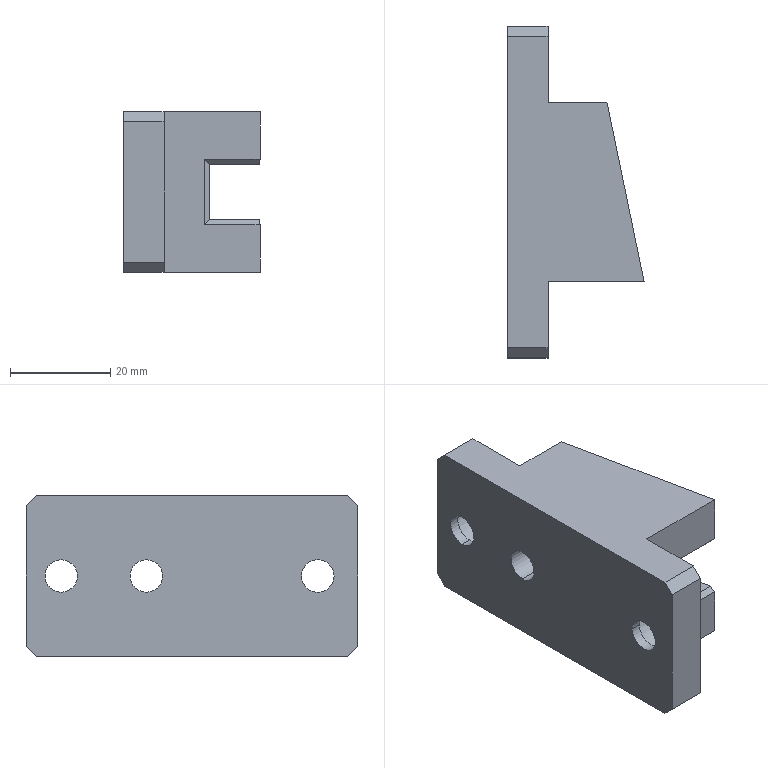Part | Creo | features CURVE 9, CUT 6, PROTRUSION 4, DATUM PLANE 3, CHAMFER 2, COORDINATE SYSTEM 1, MIRROR 1 | 1 solid | 40 faces | box 27.171 x 66.207 x 32 mm | volume 28820 mm3 | plane 28 | cylinder 12 | commonest cylinder face diameters 6.5 x6 10.5 x4 11 x2
STEP:
#1=CARTESIAN_POINT('',(0.,0.,0.));
#2=DIRECTION('',(0.,0.,1.));
#3=DIRECTION('',(1.,0.,0.));
#4=AXIS2_PLACEMENT_3D('',#1,#2,#3);
#5=CARTESIAN_POINT('',(0.,24.007,-16.));
#6=VERTEX_POINT('',#5);
#7=CARTESIAN_POINT('',(7.998,24.007,-16.));
#8=VERTEX_POINT('',#7);
#9=CARTESIAN_POINT('',(0.,24.007,-16.));
#10=DIRECTION('',(1.,0.,0.));
#11=VECTOR('',#10,7.998);
#12=LINE('',#9,#11);
#13=EDGE_CURVE('',#6,#8,#12,.T.);
#14=ORIENTED_EDGE('',*,*,#13,.F.);
#15=CARTESIAN_POINT('',(0.,-38.2,-16.));
#16=VERTEX_POINT('',#15);
#17=CARTESIAN_POINT('',(0.,24.007,-16.));
#18=DIRECTION('',(0.,-1.,0.));
#19=VECTOR('',#18,62.207);
#20=LINE('',#17,#19);
#21=EDGE_CURVE('',#6,#16,#20,.T.);
#22=ORIENTED_EDGE('',*,*,#21,.T.);
#23=CARTESIAN_POINT('',(7.998,-38.2,-16.));
#24=VERTEX_POINT('',#23);
#25=CARTESIAN_POINT('',(0.,-38.2,-16.));
#26=DIRECTION('',(1.,0.,0.));
#27=VECTOR('',#26,7.998);
#28=LINE('',#25,#27);
#29=EDGE_CURVE('',#16,#24,#28,.T.);
#30=ORIENTED_EDGE('',*,*,#29,.T.);
#31=CARTESIAN_POINT('',(7.998,-25.,-16.));
#32=VERTEX_POINT('',#31);
#33=CARTESIAN_POINT('',(7.998,-25.,-16.));
#34=DIRECTION('',(0.,-1.,0.));
#35=VECTOR('',#34,13.2);
#36=LINE('',#33,#35);
#37=EDGE_CURVE('',#32,#24,#36,.T.);
#38=ORIENTED_EDGE('',*,*,#37,.F.);
#39=CARTESIAN_POINT('',(27.171,-25.,-16.));
#40=VERTEX_POINT('',#39);
#41=CARTESIAN_POINT('',(27.171,-25.,-16.));
#42=DIRECTION('',(-1.,0.,0.));
#43=VECTOR('',#42,19.173);
#44=LINE('',#41,#43);
#45=EDGE_CURVE('',#40,#32,#44,.T.);
#46=ORIENTED_EDGE('',*,*,#45,.F.);
#47=CARTESIAN_POINT('',(19.771,10.777,-16.));
#48=VERTEX_POINT('',#47);
#49=CARTESIAN_POINT('',(27.171,-25.,-16.));
#50=DIRECTION('',(-0.2026,0.9793,0.));
#51=VECTOR('',#50,36.534);
#52=LINE('',#49,#51);
#53=EDGE_CURVE('',#40,#48,#52,.T.);
#54=ORIENTED_EDGE('',*,*,#53,.T.);
#55=CARTESIAN_POINT('',(7.998,10.777,-16.));
#56=VERTEX_POINT('',#55);
#57=CARTESIAN_POINT('',(7.998,10.777,-16.));
#58=DIRECTION('',(1.,0.,0.));
#59=VECTOR('',#58,11.773);
#60=LINE('',#57,#59);
#61=EDGE_CURVE('',#56,#48,#60,.T.);
#62=ORIENTED_EDGE('',*,*,#61,.F.);
#63=CARTESIAN_POINT('',(7.998,10.777,-16.));
#64=DIRECTION('',(0.,1.,0.));
#65=VECTOR('',#64,13.23);
#66=LINE('',#63,#65);
#67=EDGE_CURVE('',#56,#8,#66,.T.);
#68=ORIENTED_EDGE('',*,*,#67,.T.);
#69=EDGE_LOOP('',(#14,#22,#30,#38,#46,#54,#62,#68));
#70=FACE_OUTER_BOUND('',#69,.F.);
#71=CARTESIAN_POINT('',(0.,0.,-16.));
#72=DIRECTION('',(0.,0.,1.));
#73=DIRECTION('',(1.,0.,0.));
#74=AXIS2_PLACEMENT_3D('',#71,#72,#73);
#75=PLANE('',#74);
#76=ADVANCED_FACE('',(#70),#75,.F.);
#77=CARTESIAN_POINT('',(7.998,26.007,-14.));
#78=VERTEX_POINT('',#77);
#79=CARTESIAN_POINT('',(7.998,24.007,-16.));
#80=DIRECTION('',(0.,0.7071,0.7071));
#81=VECTOR('',#80,2.828);
#82=LINE('',#79,#81);
#83=EDGE_CURVE('',#8,#78,#82,.T.);
#84=ORIENTED_EDGE('',*,*,#83,.T.);
#85=CARTESIAN_POINT('',(0.,26.007,-14.));
#86=VERTEX_POINT('',#85);
#87=CARTESIAN_POINT('',(0.,26.007,-14.));
#88=DIRECTION('',(1.,0.,0.));
#89=VECTOR('',#88,7.998);
#90=LINE('',#87,#89);
#91=EDGE_CURVE('',#86,#78,#90,.T.);
#92=ORIENTED_EDGE('',*,*,#91,.F.);
#93=CARTESIAN_POINT('',(0.,26.007,-14.));
#94=DIRECTION('',(0.,-0.7071,-0.7071));
#95=VECTOR('',#94,2.828);
#96=LINE('',#93,#95);
#97=EDGE_CURVE('',#86,#6,#96,.T.);
#98=ORIENTED_EDGE('',*,*,#97,.T.);
#99=ORIENTED_EDGE('',*,*,#13,.T.);
#100=EDGE_LOOP('',(#84,#92,#98,#99));
#101=FACE_OUTER_BOUND('',#100,.F.);
#102=CARTESIAN_POINT('',(3.999,25.007,-15.));
#103=DIRECTION('',(0.,0.7071,-0.7071));
#104=DIRECTION('',(0.,0.7071,0.7071));
#105=AXIS2_PLACEMENT_3D('',#102,#103,#104);
#106=PLANE('',#105);
#107=ADVANCED_FACE('',(#101),#106,.T.);
#108=ORIENTED_EDGE('',*,*,#83,.F.);
#109=ORIENTED_EDGE('',*,*,#67,.F.);
#110=CARTESIAN_POINT('',(7.998,10.777,16.));
#111=VERTEX_POINT('',#110);
#112=CARTESIAN_POINT('',(7.998,10.777,-16.));
#113=DIRECTION('',(0.,0.,1.));
#114=VECTOR('',#113,32.);
#115=LINE('',#112,#114);
#116=EDGE_CURVE('',#56,#111,#115,.T.);
#117=ORIENTED_EDGE('',*,*,#116,.T.);
#118=CARTESIAN_POINT('',(7.998,24.007,16.));
#119=VERTEX_POINT('',#118);
#120=CARTESIAN_POINT('',(7.998,10.777,16.));
#121=DIRECTION('',(0.,1.,0.));
#122=VECTOR('',#121,13.23);
#123=LINE('',#120,#122);
#124=EDGE_CURVE('',#111,#119,#123,.T.);
#125=ORIENTED_EDGE('',*,*,#124,.T.);
#126=CARTESIAN_POINT('',(7.998,26.007,14.));
#127=VERTEX_POINT('',#126);
#128=CARTESIAN_POINT('',(7.998,26.007,14.));
#129=DIRECTION('',(0.,-0.7071,0.7071));
#130=VECTOR('',#129,2.828);
#131=LINE('',#128,#130);
#132=EDGE_CURVE('',#127,#119,#131,.T.);
#133=ORIENTED_EDGE('',*,*,#132,.F.);
#134=CARTESIAN_POINT('',(7.998,26.007,-14.));
#135=DIRECTION('',(0.,0.,1.));
#136=VECTOR('',#135,28.);
#137=LINE('',#134,#136);
#138=EDGE_CURVE('',#78,#127,#137,.T.);
#139=ORIENTED_EDGE('',*,*,#138,.F.);
#140=EDGE_LOOP('',(#108,#109,#117,#125,#133,#139));
#141=FACE_OUTER_BOUND('',#140,.F.);
#142=CARTESIAN_POINT('',(7.998,19.007,-5.25));
#143=VERTEX_POINT('',#142);
#144=CARTESIAN_POINT('',(7.998,19.007,5.25));
#145=VERTEX_POINT('',#144);
#146=CARTESIAN_POINT('',(7.998,19.007,0.));
#147=DIRECTION('',(1.,0.,0.));
#148=DIRECTION('',(0.,0.,-1.));
#149=AXIS2_PLACEMENT_3D('',#146,#147,#148);
#150=CIRCLE('',#149,5.25);
#151=EDGE_CURVE('',#143,#145,#150,.T.);
#152=ORIENTED_EDGE('',*,*,#151,.T.);
#153=CARTESIAN_POINT('',(7.998,19.007,0.));
#154=DIRECTION('',(1.,0.,0.));
#155=DIRECTION('',(0.,0.,1.));
#156=AXIS2_PLACEMENT_3D('',#153,#154,#155);
#157=CIRCLE('',#156,5.25);
#158=EDGE_CURVE('',#145,#143,#157,.T.);
#159=ORIENTED_EDGE('',*,*,#158,.T.);
#160=EDGE_LOOP('',(#152,#159));
#161=FACE_BOUND('',#160,.F.);
#162=CARTESIAN_POINT('',(7.998,10.777,-16.));
#163=DIRECTION('',(1.,0.,0.));
#164=DIRECTION('',(0.,1.,0.));
#165=AXIS2_PLACEMENT_3D('',#162,#163,#164);
#166=PLANE('',#165);
#167=ADVANCED_FACE('',(#141,#161),#166,.T.);
#168=ORIENTED_EDGE('',*,*,#151,.F.);
#169=CARTESIAN_POINT('',(1.998,19.007,-5.25));
#170=VERTEX_POINT('',#169);
#171=CARTESIAN_POINT('',(7.998,19.007,-5.25));
#172=DIRECTION('',(-1.,0.,0.));
#173=VECTOR('',#172,6.);
#174=LINE('',#171,#173);
#175=EDGE_CURVE('',#143,#170,#174,.T.);
#176=ORIENTED_EDGE('',*,*,#175,.T.);
#177=CARTESIAN_POINT('',(1.998,19.007,5.25));
#178=VERTEX_POINT('',#177);
#179=CARTESIAN_POINT('',(1.998,19.007,0.));
#180=DIRECTION('',(1.,0.,0.));
#181=DIRECTION('',(0.,0.,-1.));
#182=AXIS2_PLACEMENT_3D('',#179,#180,#181);
#183=CIRCLE('',#182,5.25);
#184=EDGE_CURVE('',#170,#178,#183,.T.);
#185=ORIENTED_EDGE('',*,*,#184,.T.);
#186=CARTESIAN_POINT('',(7.998,19.007,5.25));
#187=DIRECTION('',(-1.,0.,0.));
#188=VECTOR('',#187,6.);
#189=LINE('',#186,#188);
#190=EDGE_CURVE('',#145,#178,#189,.T.);
#191=ORIENTED_EDGE('',*,*,#190,.F.);
#192=EDGE_LOOP('',(#168,#176,#185,#191));
#193=FACE_OUTER_BOUND('',#192,.F.);
#194=CARTESIAN_POINT('',(7.998,19.007,0.));
#195=DIRECTION('',(1.,0.,0.));
#196=DIRECTION('',(0.,0.,-1.));
#197=AXIS2_PLACEMENT_3D('',#194,#195,#196);
#198=CYLINDRICAL_SURFACE('',#197,5.25);
#199=ADVANCED_FACE('',(#193),#198,.F.);
#200=ORIENTED_EDGE('',*,*,#158,.F.);
#201=ORIENTED_EDGE('',*,*,#190,.T.);
#202=CARTESIAN_POINT('',(1.998,19.007,0.));
#203=DIRECTION('',(1.,0.,0.));
#204=DIRECTION('',(0.,0.,1.));
#205=AXIS2_PLACEMENT_3D('',#202,#203,#204);
#206=CIRCLE('',#205,5.25);
#207=EDGE_CURVE('',#178,#170,#206,.T.);
#208=ORIENTED_EDGE('',*,*,#207,.T.);
#209=ORIENTED_EDGE('',*,*,#175,.F.);
#210=EDGE_LOOP('',(#200,#201,#208,#209));
#211=FACE_OUTER_BOUND('',#210,.F.);
#212=CARTESIAN_POINT('',(7.998,19.007,0.));
#213=DIRECTION('',(1.,0.,0.));
#214=DIRECTION('',(0.,0.,-1.));
#215=AXIS2_PLACEMENT_3D('',#212,#213,#214);
#216=CYLINDRICAL_SURFACE('',#215,5.25);
#217=ADVANCED_FACE('',(#211),#216,.F.);
#218=ORIENTED_EDGE('',*,*,#184,.F.);
#219=ORIENTED_EDGE('',*,*,#207,.F.);
#220=EDGE_LOOP('',(#218,#219));
#221=FACE_OUTER_BOUND('',#220,.F.);
#222=CARTESIAN_POINT('',(1.998,19.007,-3.25));
#223=VERTEX_POINT('',#222);
#224=CARTESIAN_POINT('',(1.998,19.007,3.25));
#225=VERTEX_POINT('',#224);
#226=CARTESIAN_POINT('',(1.998,19.007,0.));
#227=DIRECTION('',(1.,0.,0.));
#228=DIRECTION('',(0.,0.,-1.));
#229=AXIS2_PLACEMENT_3D('',#226,#227,#228);
#230=CIRCLE('',#229,3.25);
#231=EDGE_CURVE('',#223,#225,#230,.T.);
#232=ORIENTED_EDGE('',*,*,#231,.T.);
#233=CARTESIAN_POINT('',(1.998,19.007,0.));
#234=DIRECTION('',(1.,0.,0.));
#235=DIRECTION('',(0.,0.,1.));
#236=AXIS2_PLACEMENT_3D('',#233,#234,#235);
#237=CIRCLE('',#236,3.25);
#238=EDGE_CURVE('',#225,#223,#237,.T.);
#239=ORIENTED_EDGE('',*,*,#238,.T.);
#240=EDGE_LOOP('',(#232,#239));
#241=FACE_BOUND('',#240,.F.);
#242=CARTESIAN_POINT('',(1.998,0.,-16.));
#243=DIRECTION('',(1.,0.,0.));
#244=DIRECTION('',(0.,0.,-1.));
#245=AXIS2_PLACEMENT_3D('',#242,#243,#244);
#246=PLANE('',#245);
#247=ADVANCED_FACE('',(#221,#241),#246,.T.);
#248=ORIENTED_EDGE('',*,*,#231,.F.);
#249=CARTESIAN_POINT('',(0.,19.007,-3.25));
#250=VERTEX_POINT('',#249);
#251=CARTESIAN_POINT('',(1.998,19.007,-3.25));
#252=DIRECTION('',(-1.,0.,0.));
#253=VECTOR('',#252,1.998);
#254=LINE('',#251,#253);
#255=EDGE_CURVE('',#223,#250,#254,.T.);
#256=ORIENTED_EDGE('',*,*,#255,.T.);
#257=CARTESIAN_POINT('',(0.,19.007,3.25));
#258=VERTEX_POINT('',#257);
#259=CARTESIAN_POINT('',(0.,19.007,0.));
#260=DIRECTION('',(1.,0.,0.));
#261=DIRECTION('',(0.,0.,-1.));
#262=AXIS2_PLACEMENT_3D('',#259,#260,#261);
#263=CIRCLE('',#262,3.25);
#264=EDGE_CURVE('',#250,#258,#263,.T.);
#265=ORIENTED_EDGE('',*,*,#264,.T.);
#266=CARTESIAN_POINT('',(1.998,19.007,3.25));
#267=DIRECTION('',(-1.,0.,0.));
#268=VECTOR('',#267,1.998);
#269=LINE('',#266,#268);
#270=EDGE_CURVE('',#225,#258,#269,.T.);
#271=ORIENTED_EDGE('',*,*,#270,.F.);
#272=EDGE_LOOP('',(#248,#256,#265,#271));
#273=FACE_OUTER_BOUND('',#272,.F.);
#274=CARTESIAN_POINT('',(17.,19.007,0.));
#275=DIRECTION('',(1.,0.,0.));
#276=DIRECTION('',(0.,0.,-1.));
#277=AXIS2_PLACEMENT_3D('',#274,#275,#276);
#278=CYLINDRICAL_SURFACE('',#277,3.25);
#279=ADVANCED_FACE('',(#273),#278,.F.);
#280=ORIENTED_EDGE('',*,*,#238,.F.);
#281=ORIENTED_EDGE('',*,*,#270,.T.);
#282=CARTESIAN_POINT('',(0.,19.007,0.));
#283=DIRECTION('',(1.,0.,0.));
#284=DIRECTION('',(0.,0.,1.));
#285=AXIS2_PLACEMENT_3D('',#282,#283,#284);
#286=CIRCLE('',#285,3.25);
#287=EDGE_CURVE('',#258,#250,#286,.T.);
#288=ORIENTED_EDGE('',*,*,#287,.T.);
#289=ORIENTED_EDGE('',*,*,#255,.F.);
#290=EDGE_LOOP('',(#280,#281,#288,#289));
#291=FACE_OUTER_BOUND('',#290,.F.);
#292=CARTESIAN_POINT('',(17.,19.007,0.));
#293=DIRECTION('',(1.,0.,0.));
#294=DIRECTION('',(0.,0.,-1.));
#295=AXIS2_PLACEMENT_3D('',#292,#293,#294);
#296=CYLINDRICAL_SURFACE('',#295,3.25);
#297=ADVANCED_FACE('',(#291),#296,.F.);
#298=ORIENTED_EDGE('',*,*,#97,.F.);
#299=CARTESIAN_POINT('',(0.,26.007,14.));
#300=VERTEX_POINT('',#299);
#301=CARTESIAN_POINT('',(0.,26.007,-14.));
#302=DIRECTION('',(0.,0.,1.));
#303=VECTOR('',#302,28.);
#304=LINE('',#301,#303);
#305=EDGE_CURVE('',#86,#300,#304,.T.);
#306=ORIENTED_EDGE('',*,*,#305,.T.);
#307=CARTESIAN_POINT('',(0.,24.007,16.));
#308=VERTEX_POINT('',#307);
#309=CARTESIAN_POINT('',(0.,24.007,16.));
#310=DIRECTION('',(0.,0.7071,-0.7071));
#311=VECTOR('',#310,2.828);
#312=LINE('',#309,#311);
#313=EDGE_CURVE('',#308,#300,#312,.T.);
#314=ORIENTED_EDGE('',*,*,#313,.F.);
#315=CARTESIAN_POINT('',(0.,-38.2,16.));
#316=VERTEX_POINT('',#315);
#317=CARTESIAN_POINT('',(0.,24.007,16.));
#318=DIRECTION('',(0.,-1.,0.));
#319=VECTOR('',#318,62.207);
#320=LINE('',#317,#319);
#321=EDGE_CURVE('',#308,#316,#320,.T.);
#322=ORIENTED_EDGE('',*,*,#321,.T.);
#323=CARTESIAN_POINT('',(0.,-40.2,14.));
#324=VERTEX_POINT('',#323);
#325=CARTESIAN_POINT('',(0.,-40.2,14.));
#326=DIRECTION('',(0.,0.7071,0.7071));
#327=VECTOR('',#326,2.828);
#328=LINE('',#325,#327);
#329=EDGE_CURVE('',#324,#316,#328,.T.);
#330=ORIENTED_EDGE('',*,*,#329,.F.);
#331=CARTESIAN_POINT('',(0.,-40.2,-14.));
#332=VERTEX_POINT('',#331);
#333=CARTESIAN_POINT('',(0.,-40.2,14.));
#334=DIRECTION('',(0.,0.,-1.));
#335=VECTOR('',#334,28.);
#336=LINE('',#333,#335);
#337=EDGE_CURVE('',#324,#332,#336,.T.);
#338=ORIENTED_EDGE('',*,*,#337,.T.);
#339=CARTESIAN_POINT('',(0.,-38.2,-16.));
#340=DIRECTION('',(0.,-0.7071,0.7071));
#341=VECTOR('',#340,2.828);
#342=LINE('',#339,#341);
#343=EDGE_CURVE('',#16,#332,#342,.T.);
#344=ORIENTED_EDGE('',*,*,#343,.F.);
#345=ORIENTED_EDGE('',*,*,#21,.F.);
#346=EDGE_LOOP('',(#298,#306,#314,#322,#330,#338,#344,#345));
#347=FACE_OUTER_BOUND('',#346,.F.);
#348=CARTESIAN_POINT('',(0.,2.007,-3.25));
#349=VERTEX_POINT('',#348);
#350=CARTESIAN_POINT('',(0.,2.007,3.25));
#351=VERTEX_POINT('',#350);
#352=CARTESIAN_POINT('',(0.,2.007,0.));
#353=DIRECTION('',(1.,0.,0.));
#354=DIRECTION('',(0.,0.,-1.));
#355=AXIS2_PLACEMENT_3D('',#352,#353,#354);
#356=CIRCLE('',#355,3.25);
#357=EDGE_CURVE('',#349,#351,#356,.T.);
#358=ORIENTED_EDGE('',*,*,#357,.F.);
#359=CARTESIAN_POINT('',(0.,2.007,0.));
#360=DIRECTION('',(1.,0.,0.));
#361=DIRECTION('',(0.,0.,1.));
#362=AXIS2_PLACEMENT_3D('',#359,#360,#361);
#363=CIRCLE('',#362,3.25);
#364=EDGE_CURVE('',#351,#349,#363,.T.);
#365=ORIENTED_EDGE('',*,*,#364,.F.);
#366=EDGE_LOOP('',(#358,#365));
#367=FACE_BOUND('',#366,.F.);
#368=CARTESIAN_POINT('',(0.,-28.95,0.));
#369=VERTEX_POINT('',#368);
#370=CARTESIAN_POINT('',(0.,-35.45,0.));
#371=VERTEX_POINT('',#370);
#372=CARTESIAN_POINT('',(0.,-32.2,0.));
#373=DIRECTION('',(1.,0.,0.));
#374=DIRECTION('',(0.,1.,0.));
#375=AXIS2_PLACEMENT_3D('',#372,#373,#374);
#376=CIRCLE('',#375,3.25);
#377=EDGE_CURVE('',#369,#371,#376,.T.);
#378=ORIENTED_EDGE('',*,*,#377,.F.);
#379=CARTESIAN_POINT('',(0.,-32.2,0.));
#380=DIRECTION('',(1.,0.,0.));
#381=DIRECTION('',(0.,-1.,0.));
#382=AXIS2_PLACEMENT_3D('',#379,#380,#381);
#383=CIRCLE('',#382,3.25);
#384=EDGE_CURVE('',#371,#369,#383,.T.);
#385=ORIENTED_EDGE('',*,*,#384,.F.);
#386=EDGE_LOOP('',(#378,#385));
#387=FACE_BOUND('',#386,.F.);
#388=ORIENTED_EDGE('',*,*,#264,.F.);
#389=ORIENTED_EDGE('',*,*,#287,.F.);
#390=EDGE_LOOP('',(#388,#389));
#391=FACE_BOUND('',#390,.F.);
#392=CARTESIAN_POINT('',(0.,26.007,-16.));
#393=DIRECTION('',(-1.,0.,0.));
#394=DIRECTION('',(0.,-1.,0.));
#395=AXIS2_PLACEMENT_3D('',#392,#393,#394);
#396=PLANE('',#395);
#397=ADVANCED_FACE('',(#347,#367,#387,#391),#396,.T.);
#398=CARTESIAN_POINT('',(5.,2.007,-3.25));
#399=VERTEX_POINT('',#398);
#400=CARTESIAN_POINT('',(5.,2.007,3.25));
#401=VERTEX_POINT('',#400);
#402=CARTESIAN_POINT('',(5.,2.007,0.));
#403=DIRECTION('',(1.,0.,0.));
#404=DIRECTION('',(0.,0.,-1.));
#405=AXIS2_PLACEMENT_3D('',#402,#403,#404);
#406=CIRCLE('',#405,3.25);
#407=EDGE_CURVE('',#399,#401,#406,.T.);
#408=ORIENTED_EDGE('',*,*,#407,.F.);
#409=CARTESIAN_POINT('',(5.,2.007,-3.25));
#410=DIRECTION('',(-1.,0.,0.));
#411=VECTOR('',#410,5.);
#412=LINE('',#409,#411);
#413=EDGE_CURVE('',#399,#349,#412,.T.);
#414=ORIENTED_EDGE('',*,*,#413,.T.);
#415=ORIENTED_EDGE('',*,*,#357,.T.);
#416=CARTESIAN_POINT('',(5.,2.007,3.25));
#417=DIRECTION('',(-1.,0.,0.));
#418=VECTOR('',#417,5.);
#419=LINE('',#416,#418);
#420=EDGE_CURVE('',#401,#351,#419,.T.);
#421=ORIENTED_EDGE('',*,*,#420,.F.);
#422=EDGE_LOOP('',(#408,#414,#415,#421));
#423=FACE_OUTER_BOUND('',#422,.F.);
#424=CARTESIAN_POINT('',(17.,2.007,0.));
#425=DIRECTION('',(1.,0.,0.));
#426=DIRECTION('',(0.,0.,-1.));
#427=AXIS2_PLACEMENT_3D('',#424,#425,#426);
#428=CYLINDRICAL_SURFACE('',#427,3.25);
#429=ADVANCED_FACE('',(#423),#428,.F.);
#430=CARTESIAN_POINT('',(5.,2.007,-5.25));
#431=VERTEX_POINT('',#430);
#432=CARTESIAN_POINT('',(5.,2.007,5.25));
#433=VERTEX_POINT('',#432);
#434=CARTESIAN_POINT('',(5.,2.007,0.));
#435=DIRECTION('',(1.,0.,0.));
#436=DIRECTION('',(0.,0.,-1.));
#437=AXIS2_PLACEMENT_3D('',#434,#435,#436);
#438=CIRCLE('',#437,5.25);
#439=EDGE_CURVE('',#431,#433,#438,.T.);
#440=ORIENTED_EDGE('',*,*,#439,.F.);
#441=CARTESIAN_POINT('',(5.,2.007,0.));
#442=DIRECTION('',(1.,0.,0.));
#443=DIRECTION('',(0.,0.,1.));
#444=AXIS2_PLACEMENT_3D('',#441,#442,#443);
#445=CIRCLE('',#444,5.25);
#446=EDGE_CURVE('',#433,#431,#445,.T.);
#447=ORIENTED_EDGE('',*,*,#446,.F.);
#448=EDGE_LOOP('',(#440,#447));
#449=FACE_OUTER_BOUND('',#448,.F.);
#450=ORIENTED_EDGE('',*,*,#407,.T.);
#451=CARTESIAN_POINT('',(5.,2.007,0.));
#452=DIRECTION('',(1.,0.,0.));
#453=DIRECTION('',(0.,0.,1.));
#454=AXIS2_PLACEMENT_3D('',#451,#452,#453);
#455=CIRCLE('',#454,3.25);
#456=EDGE_CURVE('',#401,#399,#455,.T.);
#457=ORIENTED_EDGE('',*,*,#456,.T.);
#458=EDGE_LOOP('',(#450,#457));
#459=FACE_BOUND('',#458,.F.);
#460=CARTESIAN_POINT('',(5.,0.,5.5));
#461=DIRECTION('',(1.,0.,0.));
#462=DIRECTION('',(0.,0.,-1.));
#463=AXIS2_PLACEMENT_3D('',#460,#461,#462);
#464=PLANE('',#463);
#465=ADVANCED_FACE('',(#449,#459),#464,.T.);
#466=CARTESIAN_POINT('',(11.96,2.007,-5.25));
#467=VERTEX_POINT('',#466);
#468=CARTESIAN_POINT('',(11.96,2.007,5.25));
#469=VERTEX_POINT('',#468);
#470=CARTESIAN_POINT('',(11.821,2.626,-5.25));
#471=CARTESIAN_POINT('',(11.522,3.963,-5.026));
#472=CARTESIAN_POINT('',(11.174,5.517,-4.024));
#473=CARTESIAN_POINT('',(10.969,6.434,-2.889));
#474=CARTESIAN_POINT('',(10.86,6.923,-1.939));
#475=CARTESIAN_POINT('',(10.798,7.202,-0.9481));
#476=CARTESIAN_POINT('',(10.779,7.284,0.));
#477=CARTESIAN_POINT('',(10.798,7.202,0.9481));
#478=CARTESIAN_POINT('',(10.86,6.923,1.939));
#479=CARTESIAN_POINT('',(10.969,6.434,2.889));
#480=CARTESIAN_POINT('',(11.174,5.517,4.024));
#481=CARTESIAN_POINT('',(11.522,3.963,5.026));
#482=CARTESIAN_POINT('',(11.821,2.626,5.25));
#483=B_SPLINE_CURVE_WITH_KNOTS('',3,(#466,#470,#471,#472,#473,#474,#475,#476,#477,#478,#479,#480,#481,#482,#468),.UNSPECIFIED.,.F.,.F.,(4,1,1,1,1,1,1,1,1,1,1,1,4),(0.,0.125,0.25,0.3125,0.375,0.4375,0.5,0.5625,0.625,0.6875,0.75,0.875,1.),.UNSPECIFIED.);
#484=EDGE_CURVE('',#467,#469,#483,.T.);
#485=ORIENTED_EDGE('',*,*,#484,.F.);
#486=CARTESIAN_POINT('',(11.96,2.007,-5.25));
#487=DIRECTION('',(-1.,0.,0.));
#488=VECTOR('',#487,6.96);
#489=LINE('',#486,#488);
#490=EDGE_CURVE('',#467,#431,#489,.T.);
#491=ORIENTED_EDGE('',*,*,#490,.T.);
#492=ORIENTED_EDGE('',*,*,#439,.T.);
#493=CARTESIAN_POINT('',(11.96,2.007,5.25));
#494=DIRECTION('',(-1.,0.,0.));
#495=VECTOR('',#494,6.96);
#496=LINE('',#493,#495);
#497=EDGE_CURVE('',#469,#433,#496,.T.);
#498=ORIENTED_EDGE('',*,*,#497,.F.);
#499=EDGE_LOOP('',(#485,#491,#492,#498));
#500=FACE_OUTER_BOUND('',#499,.F.);
#501=CARTESIAN_POINT('',(17.,2.007,0.));
#502=DIRECTION('',(1.,0.,0.));
#503=DIRECTION('',(0.,0.,-1.));
#504=AXIS2_PLACEMENT_3D('',#501,#502,#503);
#505=CYLINDRICAL_SURFACE('',#504,5.25);
#506=ADVANCED_FACE('',(#500),#505,.F.);
#507=CARTESIAN_POINT('',(10.216,9.801,5.524));
#508=VERTEX_POINT('',#507);
#509=CARTESIAN_POINT('',(10.216,9.801,-5.524));
#510=VERTEX_POINT('',#509);
#511=CARTESIAN_POINT('',(10.216,9.801,5.524));
#512=DIRECTION('',(0.,0.,-1.));
#513=VECTOR('',#512,11.048);
#514=LINE('',#511,#513);
#515=EDGE_CURVE('',#508,#510,#514,.T.);
#516=ORIENTED_EDGE('',*,*,#515,.T.);
#517=CARTESIAN_POINT('',(10.222,9.777,-5.5));
#518=VERTEX_POINT('',#517);
#519=CARTESIAN_POINT('',(10.222,9.777,-5.5));
#520=DIRECTION('',(-0.1562,0.6984,-0.6984));
#521=VECTOR('',#520,0.03452);
#522=LINE('',#519,#521);
#523=EDGE_CURVE('',#518,#510,#522,.T.);
#524=ORIENTED_EDGE('',*,*,#523,.F.);
#525=CARTESIAN_POINT('',(17.,-20.529,-5.5));
#526=VERTEX_POINT('',#525);
#527=CARTESIAN_POINT('',(10.222,9.777,-5.5));
#528=DIRECTION('',(0.2183,-0.9759,0.));
#529=VECTOR('',#528,31.055);
#530=LINE('',#527,#529);
#531=EDGE_CURVE('',#518,#526,#530,.T.);
#532=ORIENTED_EDGE('',*,*,#531,.T.);
#533=CARTESIAN_POINT('',(17.,-20.529,5.5));
#534=VERTEX_POINT('',#533);
#535=CARTESIAN_POINT('',(17.,-20.529,5.5));
#536=DIRECTION('',(0.,0.,-1.));
#537=VECTOR('',#536,11.);
#538=LINE('',#535,#537);
#539=EDGE_CURVE('',#534,#526,#538,.T.);
#540=ORIENTED_EDGE('',*,*,#539,.F.);
#541=CARTESIAN_POINT('',(10.222,9.777,5.5));
#542=VERTEX_POINT('',#541);
#543=CARTESIAN_POINT('',(10.222,9.777,5.5));
#544=DIRECTION('',(0.2183,-0.9759,0.));
#545=VECTOR('',#544,31.055);
#546=LINE('',#543,#545);
#547=EDGE_CURVE('',#542,#534,#546,.T.);
#548=ORIENTED_EDGE('',*,*,#547,.F.);
#549=CARTESIAN_POINT('',(10.216,9.801,5.524));
#550=DIRECTION('',(0.1562,-0.6984,-0.6984));
#551=VECTOR('',#550,0.03452);
#552=LINE('',#549,#551);
#553=EDGE_CURVE('',#508,#542,#552,.T.);
#554=ORIENTED_EDGE('',*,*,#553,.F.);
#555=EDGE_LOOP('',(#516,#524,#532,#540,#548,#554));
#556=FACE_OUTER_BOUND('',#555,.F.);
#557=ORIENTED_EDGE('',*,*,#484,.T.);
#558=CARTESIAN_POINT('',(11.96,2.007,5.25));
#559=CARTESIAN_POINT('',(12.098,1.388,5.25));
#560=CARTESIAN_POINT('',(12.397,0.05091,5.026));
#561=CARTESIAN_POINT('',(12.745,-1.503,4.024));
#562=CARTESIAN_POINT('',(12.95,-2.42,2.889));
#563=CARTESIAN_POINT('',(13.059,-2.91,1.939));
#564=CARTESIAN_POINT('',(13.121,-3.188,0.9481));
#565=CARTESIAN_POINT('',(13.14,-3.271,0.));
#566=CARTESIAN_POINT('',(13.121,-3.188,-0.9481));
#567=CARTESIAN_POINT('',(13.059,-2.91,-1.939));
#568=CARTESIAN_POINT('',(12.95,-2.42,-2.889));
#569=CARTESIAN_POINT('',(12.745,-1.503,-4.024));
#570=CARTESIAN_POINT('',(12.397,0.05091,-5.026));
#571=CARTESIAN_POINT('',(12.098,1.388,-5.25));
#572=CARTESIAN_POINT('',(11.96,2.007,-5.25));
#573=B_SPLINE_CURVE_WITH_KNOTS('',3,(#558,#559,#560,#561,#562,#563,#564,#565,#566,#567,#568,#569,#570,#571,#572),.UNSPECIFIED.,.F.,.F.,(4,1,1,1,1,1,1,1,1,1,1,1,4),(0.,0.125,0.25,0.3125,0.375,0.4375,0.5,0.5625,0.625,0.6875,0.75,0.875,1.),.UNSPECIFIED.);
#574=EDGE_CURVE('',#469,#467,#573,.T.);
#575=ORIENTED_EDGE('',*,*,#574,.T.);
#576=EDGE_LOOP('',(#557,#575));
#577=FACE_BOUND('',#576,.F.);
#578=CARTESIAN_POINT('',(9.998,10.777,5.5));
#579=DIRECTION('',(-0.9759,-0.2183,0.));
#580=DIRECTION('',(0.2183,-0.9759,0.));
#581=AXIS2_PLACEMENT_3D('',#578,#579,#580);
#582=PLANE('',#581);
#583=ADVANCED_FACE('',(#556,#577),#582,.F.);
#584=ORIENTED_EDGE('',*,*,#574,.F.);
#585=ORIENTED_EDGE('',*,*,#497,.T.);
#586=ORIENTED_EDGE('',*,*,#446,.T.);
#587=ORIENTED_EDGE('',*,*,#490,.F.);
#588=EDGE_LOOP('',(#584,#585,#586,#587));
#589=FACE_OUTER_BOUND('',#588,.F.);
#590=CARTESIAN_POINT('',(17.,2.007,0.));
#591=DIRECTION('',(1.,0.,0.));
#592=DIRECTION('',(0.,0.,-1.));
#593=AXIS2_PLACEMENT_3D('',#590,#591,#592);
#594=CYLINDRICAL_SURFACE('',#593,5.25);
#595=ADVANCED_FACE('',(#589),#594,.F.);
#596=ORIENTED_EDGE('',*,*,#515,.F.);
#597=CARTESIAN_POINT('',(8.998,10.777,6.5));
#598=VERTEX_POINT('',#597);
#599=CARTESIAN_POINT('',(10.216,9.801,5.524));
#600=DIRECTION('',(-0.6618,0.5301,0.5301));
#601=VECTOR('',#600,1.841);
#602=LINE('',#599,#601);
#603=EDGE_CURVE('',#508,#598,#602,.T.);
#604=ORIENTED_EDGE('',*,*,#603,.T.);
#605=CARTESIAN_POINT('',(8.998,10.777,-6.5));
#606=VERTEX_POINT('',#605);
#607=CARTESIAN_POINT('',(8.998,10.777,6.5));
#608=DIRECTION('',(0.,0.,-1.));
#609=VECTOR('',#608,13.);
#610=LINE('',#607,#609);
#611=EDGE_CURVE('',#598,#606,#610,.T.);
#612=ORIENTED_EDGE('',*,*,#611,.T.);
#613=CARTESIAN_POINT('',(10.216,9.801,-5.524));
#614=DIRECTION('',(-0.6618,0.5301,-0.5301));
#615=VECTOR('',#614,1.841);
#616=LINE('',#613,#615);
#617=EDGE_CURVE('',#510,#606,#616,.T.);
#618=ORIENTED_EDGE('',*,*,#617,.F.);
#619=EDGE_LOOP('',(#596,#604,#612,#618));
#620=FACE_OUTER_BOUND('',#619,.F.);
#621=CARTESIAN_POINT('',(9.607,10.289,0.));
#622=DIRECTION('',(0.6252,0.7805,0.));
#623=DIRECTION('',(0.7805,-0.6252,0.));
#624=AXIS2_PLACEMENT_3D('',#621,#622,#623);
#625=PLANE('',#624);
#626=ADVANCED_FACE('',(#620),#625,.T.);
#627=CARTESIAN_POINT('',(19.977,9.777,5.5));
#628=VERTEX_POINT('',#627);
#629=CARTESIAN_POINT('',(19.771,10.777,6.5));
#630=VERTEX_POINT('',#629);
#631=CARTESIAN_POINT('',(19.977,9.777,5.5));
#632=DIRECTION('',(-0.1447,0.6997,0.6997));
#633=VECTOR('',#632,1.429);
#634=LINE('',#631,#633);
#635=EDGE_CURVE('',#628,#630,#634,.T.);
#636=ORIENTED_EDGE('',*,*,#635,.T.);
#637=CARTESIAN_POINT('',(19.771,10.777,6.5));
#638=DIRECTION('',(-1.,0.,0.));
#639=VECTOR('',#638,10.773);
#640=LINE('',#637,#639);
#641=EDGE_CURVE('',#630,#598,#640,.T.);
#642=ORIENTED_EDGE('',*,*,#641,.T.);
#643=ORIENTED_EDGE('',*,*,#603,.F.);
#644=ORIENTED_EDGE('',*,*,#553,.T.);
#645=CARTESIAN_POINT('',(19.977,9.777,5.5));
#646=DIRECTION('',(-1.,0.,0.));
#647=VECTOR('',#646,9.756);
#648=LINE('',#645,#647);
#649=EDGE_CURVE('',#628,#542,#648,.T.);
#650=ORIENTED_EDGE('',*,*,#649,.F.);
#651=EDGE_LOOP('',(#636,#642,#643,#644,#650));
#652=FACE_OUTER_BOUND('',#651,.F.);
#653=CARTESIAN_POINT('',(14.996,10.277,6.));
#654=DIRECTION('',(0.,0.7071,-0.7071));
#655=DIRECTION('',(0.,-0.7071,-0.7071));
#656=AXIS2_PLACEMENT_3D('',#653,#654,#655);
#657=PLANE('',#656);
#658=ADVANCED_FACE('',(#652),#657,.T.);
#659=CARTESIAN_POINT('',(27.171,-25.,6.5));
#660=VERTEX_POINT('',#659);
#661=CARTESIAN_POINT('',(26.964,-24.,5.5));
#662=VERTEX_POINT('',#661);
#663=CARTESIAN_POINT('',(27.171,-25.,6.5));
#664=DIRECTION('',(-0.1447,0.6997,-0.6997));
#665=VECTOR('',#664,1.429);
#666=LINE('',#663,#665);
#667=EDGE_CURVE('',#660,#662,#666,.T.);
#668=ORIENTED_EDGE('',*,*,#667,.F.);
#669=CARTESIAN_POINT('',(27.171,-25.,16.));
#670=VERTEX_POINT('',#669);
#671=CARTESIAN_POINT('',(27.171,-25.,16.));
#672=DIRECTION('',(0.,0.,-1.));
#673=VECTOR('',#672,9.5);
#674=LINE('',#671,#673);
#675=EDGE_CURVE('',#670,#660,#674,.T.);
#676=ORIENTED_EDGE('',*,*,#675,.F.);
#677=CARTESIAN_POINT('',(19.771,10.777,16.));
#678=VERTEX_POINT('',#677);
#679=CARTESIAN_POINT('',(27.171,-25.,16.));
#680=DIRECTION('',(-0.2026,0.9793,0.));
#681=VECTOR('',#680,36.534);
#682=LINE('',#679,#681);
#683=EDGE_CURVE('',#670,#678,#682,.T.);
#684=ORIENTED_EDGE('',*,*,#683,.T.);
#685=CARTESIAN_POINT('',(19.771,10.777,16.));
#686=DIRECTION('',(0.,0.,-1.));
#687=VECTOR('',#686,9.5);
#688=LINE('',#685,#687);
#689=EDGE_CURVE('',#678,#630,#688,.T.);
#690=ORIENTED_EDGE('',*,*,#689,.T.);
#691=ORIENTED_EDGE('',*,*,#635,.F.);
#692=CARTESIAN_POINT('',(26.964,-24.,5.5));
#693=DIRECTION('',(-0.2026,0.9793,0.));
#694=VECTOR('',#693,34.492);
#695=LINE('',#692,#694);
#696=EDGE_CURVE('',#662,#628,#695,.T.);
#697=ORIENTED_EDGE('',*,*,#696,.F.);
#698=EDGE_LOOP('',(#668,#676,#684,#690,#691,#697));
#699=FACE_OUTER_BOUND('',#698,.F.);
#700=CARTESIAN_POINT('',(27.171,-25.,16.));
#701=DIRECTION('',(0.9793,0.2026,0.));
#702=DIRECTION('',(-0.2026,0.9793,0.));
#703=AXIS2_PLACEMENT_3D('',#700,#701,#702);
#704=PLANE('',#703);
#705=ADVANCED_FACE('',(#699),#704,.T.);
#706=ORIENTED_EDGE('',*,*,#667,.T.);
#707=CARTESIAN_POINT('',(17.,-24.,5.5));
#708=VERTEX_POINT('',#707);
#709=CARTESIAN_POINT('',(17.,-24.,5.5));
#710=DIRECTION('',(1.,0.,0.));
#711=VECTOR('',#710,9.964);
#712=LINE('',#709,#711);
#713=EDGE_CURVE('',#708,#662,#712,.T.);
#714=ORIENTED_EDGE('',*,*,#713,.F.);
#715=CARTESIAN_POINT('',(16.,-25.,6.5));
#716=VERTEX_POINT('',#715);
#717=CARTESIAN_POINT('',(17.,-24.,5.5));
#718=DIRECTION('',(-0.5774,-0.5774,0.5774));
#719=VECTOR('',#718,1.732);
#720=LINE('',#717,#719);
#721=EDGE_CURVE('',#708,#716,#720,.T.);
#722=ORIENTED_EDGE('',*,*,#721,.T.);
#723=CARTESIAN_POINT('',(16.,-25.,6.5));
#724=DIRECTION('',(1.,0.,0.));
#725=VECTOR('',#724,11.171);
#726=LINE('',#723,#725);
#727=EDGE_CURVE('',#716,#660,#726,.T.);
#728=ORIENTED_EDGE('',*,*,#727,.T.);
#729=EDGE_LOOP('',(#706,#714,#722,#728));
#730=FACE_OUTER_BOUND('',#729,.F.);
#731=CARTESIAN_POINT('',(21.982,-24.5,6.));
#732=DIRECTION('',(0.,-0.7071,-0.7071));
#733=DIRECTION('',(0.,0.7071,-0.7071));
#734=AXIS2_PLACEMENT_3D('',#731,#732,#733);
#735=PLANE('',#734);
#736=ADVANCED_FACE('',(#730),#735,.T.);
#737=ORIENTED_EDGE('',*,*,#713,.T.);
#738=ORIENTED_EDGE('',*,*,#696,.T.);
#739=ORIENTED_EDGE('',*,*,#649,.T.);
#740=ORIENTED_EDGE('',*,*,#547,.T.);
#741=CARTESIAN_POINT('',(17.,-20.529,5.5));
#742=DIRECTION('',(0.,-1.,0.));
#743=VECTOR('',#742,3.471);
#744=LINE('',#741,#743);
#745=EDGE_CURVE('',#534,#708,#744,.T.);
#746=ORIENTED_EDGE('',*,*,#745,.T.);
#747=EDGE_LOOP('',(#737,#738,#739,#740,#746));
#748=FACE_OUTER_BOUND('',#747,.F.);
#749=CARTESIAN_POINT('',(0.,0.,5.5));
#750=DIRECTION('',(0.,0.,1.));
#751=DIRECTION('',(1.,0.,0.));
#752=AXIS2_PLACEMENT_3D('',#749,#750,#751);
#753=PLANE('',#752);
#754=ADVANCED_FACE('',(#748),#753,.F.);
#755=CARTESIAN_POINT('',(17.,-24.,-5.5));
#756=VERTEX_POINT('',#755);
#757=CARTESIAN_POINT('',(17.,-24.,-5.5));
#758=DIRECTION('',(0.,0.,1.));
#759=VECTOR('',#758,11.);
#760=LINE('',#757,#759);
#761=EDGE_CURVE('',#756,#708,#760,.T.);
#762=ORIENTED_EDGE('',*,*,#761,.T.);
#763=ORIENTED_EDGE('',*,*,#745,.F.);
#764=ORIENTED_EDGE('',*,*,#539,.T.);
#765=CARTESIAN_POINT('',(17.,-20.529,-5.5));
#766=DIRECTION('',(0.,-1.,0.));
#767=VECTOR('',#766,3.471);
#768=LINE('',#765,#767);
#769=EDGE_CURVE('',#526,#756,#768,.T.);
#770=ORIENTED_EDGE('',*,*,#769,.T.);
#771=EDGE_LOOP('',(#762,#763,#764,#770));
#772=FACE_OUTER_BOUND('',#771,.F.);
#773=CARTESIAN_POINT('',(17.,-20.529,5.5));
#774=DIRECTION('',(-1.,0.,0.));
#775=DIRECTION('',(0.,-1.,0.));
#776=AXIS2_PLACEMENT_3D('',#773,#774,#775);
#777=PLANE('',#776);
#778=ADVANCED_FACE('',(#772),#777,.F.);
#779=CARTESIAN_POINT('',(16.,-25.,-6.5));
#780=VERTEX_POINT('',#779);
#781=CARTESIAN_POINT('',(16.,-25.,-6.5));
#782=DIRECTION('',(0.,0.,1.));
#783=VECTOR('',#782,13.);
#784=LINE('',#781,#783);
#785=EDGE_CURVE('',#780,#716,#784,.T.);
#786=ORIENTED_EDGE('',*,*,#785,.T.);
#787=ORIENTED_EDGE('',*,*,#721,.F.);
#788=ORIENTED_EDGE('',*,*,#761,.F.);
#789=CARTESIAN_POINT('',(17.,-24.,-5.5));
#790=DIRECTION('',(-0.5774,-0.5774,-0.5774));
#791=VECTOR('',#790,1.732);
#792=LINE('',#789,#791);
#793=EDGE_CURVE('',#756,#780,#792,.T.);
#794=ORIENTED_EDGE('',*,*,#793,.T.);
#795=EDGE_LOOP('',(#786,#787,#788,#794));
#796=FACE_OUTER_BOUND('',#795,.F.);
#797=CARTESIAN_POINT('',(16.5,-24.5,0.));
#798=DIRECTION('',(0.7071,-0.7071,0.));
#799=DIRECTION('',(0.7071,0.7071,0.));
#800=AXIS2_PLACEMENT_3D('',#797,#798,#799);
#801=PLANE('',#800);
#802=ADVANCED_FACE('',(#796),#801,.T.);
#803=CARTESIAN_POINT('',(7.998,-25.,16.));
#804=VERTEX_POINT('',#803);
#805=CARTESIAN_POINT('',(7.998,-25.,-16.));
#806=DIRECTION('',(0.,0.,1.));
#807=VECTOR('',#806,32.);
#808=LINE('',#805,#807);
#809=EDGE_CURVE('',#32,#804,#808,.T.);
#810=ORIENTED_EDGE('',*,*,#809,.T.);
#811=CARTESIAN_POINT('',(7.998,-25.,16.));
#812=DIRECTION('',(1.,0.,0.));
#813=VECTOR('',#812,19.173);
#814=LINE('',#811,#813);
#815=EDGE_CURVE('',#804,#670,#814,.T.);
#816=ORIENTED_EDGE('',*,*,#815,.T.);
#817=ORIENTED_EDGE('',*,*,#675,.T.);
#818=ORIENTED_EDGE('',*,*,#727,.F.);
#819=ORIENTED_EDGE('',*,*,#785,.F.);
#820=CARTESIAN_POINT('',(27.171,-25.,-6.5));
#821=VERTEX_POINT('',#820);
#822=CARTESIAN_POINT('',(27.171,-25.,-6.5));
#823=DIRECTION('',(-1.,0.,0.));
#824=VECTOR('',#823,11.171);
#825=LINE('',#822,#824);
#826=EDGE_CURVE('',#821,#780,#825,.T.);
#827=ORIENTED_EDGE('',*,*,#826,.F.);
#828=CARTESIAN_POINT('',(27.171,-25.,-16.));
#829=DIRECTION('',(0.,0.,1.));
#830=VECTOR('',#829,9.5);
#831=LINE('',#828,#830);
#832=EDGE_CURVE('',#40,#821,#831,.T.);
#833=ORIENTED_EDGE('',*,*,#832,.F.);
#834=ORIENTED_EDGE('',*,*,#45,.T.);
#835=EDGE_LOOP('',(#810,#816,#817,#818,#819,#827,#833,#834));
#836=FACE_OUTER_BOUND('',#835,.F.);
#837=CARTESIAN_POINT('',(0.,-25.,-16.));
#838=DIRECTION('',(0.,-1.,0.));
#839=DIRECTION('',(1.,0.,0.));
#840=AXIS2_PLACEMENT_3D('',#837,#838,#839);
#841=PLANE('',#840);
#842=ADVANCED_FACE('',(#836),#841,.T.);
#843=CARTESIAN_POINT('',(7.998,-38.2,16.));
#844=VERTEX_POINT('',#843);
#845=CARTESIAN_POINT('',(7.998,-40.2,14.));
#846=VERTEX_POINT('',#845);
#847=CARTESIAN_POINT('',(7.998,-38.2,16.));
#848=DIRECTION('',(0.,-0.7071,-0.7071));
#849=VECTOR('',#848,2.828);
#850=LINE('',#847,#849);
#851=EDGE_CURVE('',#844,#846,#850,.T.);
#852=ORIENTED_EDGE('',*,*,#851,.F.);
#853=CARTESIAN_POINT('',(7.998,-25.,16.));
#854=DIRECTION('',(0.,-1.,0.));
#855=VECTOR('',#854,13.2);
#856=LINE('',#853,#855);
#857=EDGE_CURVE('',#804,#844,#856,.T.);
#858=ORIENTED_EDGE('',*,*,#857,.F.);
#859=ORIENTED_EDGE('',*,*,#809,.F.);
#860=ORIENTED_EDGE('',*,*,#37,.T.);
#861=CARTESIAN_POINT('',(7.998,-40.2,-14.));
#862=VERTEX_POINT('',#861);
#863=CARTESIAN_POINT('',(7.998,-40.2,-14.));
#864=DIRECTION('',(0.,0.7071,-0.7071));
#865=VECTOR('',#864,2.828);
#866=LINE('',#863,#865);
#867=EDGE_CURVE('',#862,#24,#866,.T.);
#868=ORIENTED_EDGE('',*,*,#867,.F.);
#869=CARTESIAN_POINT('',(7.998,-40.2,-14.));
#870=DIRECTION('',(0.,0.,1.));
#871=VECTOR('',#870,28.);
#872=LINE('',#869,#871);
#873=EDGE_CURVE('',#862,#846,#872,.T.);
#874=ORIENTED_EDGE('',*,*,#873,.T.);
#875=EDGE_LOOP('',(#852,#858,#859,#860,#868,#874));
#876=FACE_OUTER_BOUND('',#875,.F.);
#877=CARTESIAN_POINT('',(7.998,-26.7,0.));
#878=VERTEX_POINT('',#877);
#879=CARTESIAN_POINT('',(7.998,-37.7,0.));
#880=VERTEX_POINT('',#879);
#881=CARTESIAN_POINT('',(7.998,-32.2,0.));
#882=DIRECTION('',(1.,0.,0.));
#883=DIRECTION('',(0.,1.,0.));
#884=AXIS2_PLACEMENT_3D('',#881,#882,#883);
#885=CIRCLE('',#884,5.5);
#886=EDGE_CURVE('',#878,#880,#885,.T.);
#887=ORIENTED_EDGE('',*,*,#886,.T.);
#888=CARTESIAN_POINT('',(7.998,-32.2,0.));
#889=DIRECTION('',(1.,0.,0.));
#890=DIRECTION('',(0.,-1.,0.));
#891=AXIS2_PLACEMENT_3D('',#888,#889,#890);
#892=CIRCLE('',#891,5.5);
#893=EDGE_CURVE('',#880,#878,#892,.T.);
#894=ORIENTED_EDGE('',*,*,#893,.T.);
#895=EDGE_LOOP('',(#887,#894));
#896=FACE_BOUND('',#895,.F.);
#897=CARTESIAN_POINT('',(7.998,-25.,-16.));
#898=DIRECTION('',(1.,0.,0.));
#899=DIRECTION('',(0.,0.,1.));
#900=AXIS2_PLACEMENT_3D('',#897,#898,#899);
#901=PLANE('',#900);
#902=ADVANCED_FACE('',(#876,#896),#901,.T.);
#903=ORIENTED_EDGE('',*,*,#886,.F.);
#904=CARTESIAN_POINT('',(1.998,-26.7,0.));
#905=VERTEX_POINT('',#904);
#906=CARTESIAN_POINT('',(7.998,-26.7,0.));
#907=DIRECTION('',(-1.,0.,0.));
#908=VECTOR('',#907,6.);
#909=LINE('',#906,#908);
#910=EDGE_CURVE('',#878,#905,#909,.T.);
#911=ORIENTED_EDGE('',*,*,#910,.T.);
#912=CARTESIAN_POINT('',(1.998,-37.7,0.));
#913=VERTEX_POINT('',#912);
#914=CARTESIAN_POINT('',(1.998,-32.2,0.));
#915=DIRECTION('',(1.,0.,0.));
#916=DIRECTION('',(0.,1.,0.));
#917=AXIS2_PLACEMENT_3D('',#914,#915,#916);
#918=CIRCLE('',#917,5.5);
#919=EDGE_CURVE('',#905,#913,#918,.T.);
#920=ORIENTED_EDGE('',*,*,#919,.T.);
#921=CARTESIAN_POINT('',(7.998,-37.7,0.));
#922=DIRECTION('',(-1.,0.,0.));
#923=VECTOR('',#922,6.);
#924=LINE('',#921,#923);
#925=EDGE_CURVE('',#880,#913,#924,.T.);
#926=ORIENTED_EDGE('',*,*,#925,.F.);
#927=EDGE_LOOP('',(#903,#911,#920,#926));
#928=FACE_OUTER_BOUND('',#927,.F.);
#929=CARTESIAN_POINT('',(7.998,-32.2,0.));
#930=DIRECTION('',(1.,0.,0.));
#931=DIRECTION('',(0.,1.,0.));
#932=AXIS2_PLACEMENT_3D('',#929,#930,#931);
#933=CYLINDRICAL_SURFACE('',#932,5.5);
#934=ADVANCED_FACE('',(#928),#933,.F.);
#935=ORIENTED_EDGE('',*,*,#893,.F.);
#936=ORIENTED_EDGE('',*,*,#925,.T.);
#937=CARTESIAN_POINT('',(1.998,-32.2,0.));
#938=DIRECTION('',(1.,0.,0.));
#939=DIRECTION('',(0.,-1.,0.));
#940=AXIS2_PLACEMENT_3D('',#937,#938,#939);
#941=CIRCLE('',#940,5.5);
#942=EDGE_CURVE('',#913,#905,#941,.T.);
#943=ORIENTED_EDGE('',*,*,#942,.T.);
#944=ORIENTED_EDGE('',*,*,#910,.F.);
#945=EDGE_LOOP('',(#935,#936,#943,#944));
#946=FACE_OUTER_BOUND('',#945,.F.);
#947=CARTESIAN_POINT('',(7.998,-32.2,0.));
#948=DIRECTION('',(1.,0.,0.));
#949=DIRECTION('',(0.,1.,0.));
#950=AXIS2_PLACEMENT_3D('',#947,#948,#949);
#951=CYLINDRICAL_SURFACE('',#950,5.5);
#952=ADVANCED_FACE('',(#946),#951,.F.);
#953=ORIENTED_EDGE('',*,*,#919,.F.);
#954=ORIENTED_EDGE('',*,*,#942,.F.);
#955=EDGE_LOOP('',(#953,#954));
#956=FACE_OUTER_BOUND('',#955,.F.);
#957=CARTESIAN_POINT('',(1.998,-28.95,0.));
#958=VERTEX_POINT('',#957);
#959=CARTESIAN_POINT('',(1.998,-35.45,0.));
#960=VERTEX_POINT('',#959);
#961=CARTESIAN_POINT('',(1.998,-32.2,0.));
#962=DIRECTION('',(1.,0.,0.));
#963=DIRECTION('',(0.,1.,0.));
#964=AXIS2_PLACEMENT_3D('',#961,#962,#963);
#965=CIRCLE('',#964,3.25);
#966=EDGE_CURVE('',#958,#960,#965,.T.);
#967=ORIENTED_EDGE('',*,*,#966,.T.);
#968=CARTESIAN_POINT('',(1.998,-32.2,0.));
#969=DIRECTION('',(1.,0.,0.));
#970=DIRECTION('',(0.,-1.,0.));
#971=AXIS2_PLACEMENT_3D('',#968,#969,#970);
#972=CIRCLE('',#971,3.25);
#973=EDGE_CURVE('',#960,#958,#972,.T.);
#974=ORIENTED_EDGE('',*,*,#973,.T.);
#975=EDGE_LOOP('',(#967,#974));
#976=FACE_BOUND('',#975,.F.);
#977=CARTESIAN_POINT('',(1.998,-40.2,-16.));
#978=DIRECTION('',(1.,0.,0.));
#979=DIRECTION('',(0.,1.,0.));
#980=AXIS2_PLACEMENT_3D('',#977,#978,#979);
#981=PLANE('',#980);
#982=ADVANCED_FACE('',(#956,#976),#981,.T.);
#983=ORIENTED_EDGE('',*,*,#377,.T.);
#984=CARTESIAN_POINT('',(1.998,-35.45,0.));
#985=DIRECTION('',(-1.,0.,0.));
#986=VECTOR('',#985,1.998);
#987=LINE('',#984,#986);
#988=EDGE_CURVE('',#960,#371,#987,.T.);
#989=ORIENTED_EDGE('',*,*,#988,.F.);
#990=ORIENTED_EDGE('',*,*,#966,.F.);
#991=CARTESIAN_POINT('',(1.998,-28.95,0.));
#992=DIRECTION('',(-1.,0.,0.));
#993=VECTOR('',#992,1.998);
#994=LINE('',#991,#993);
#995=EDGE_CURVE('',#958,#369,#994,.T.);
#996=ORIENTED_EDGE('',*,*,#995,.T.);
#997=EDGE_LOOP('',(#983,#989,#990,#996));
#998=FACE_OUTER_BOUND('',#997,.F.);
#999=CARTESIAN_POINT('',(7.998,-32.2,0.));
#1000=DIRECTION('',(1.,0.,0.));
#1001=DIRECTION('',(0.,1.,0.));
#1002=AXIS2_PLACEMENT_3D('',#999,#1000,#1001);
#1003=CYLINDRICAL_SURFACE('',#1002,3.25);
#1004=ADVANCED_FACE('',(#998),#1003,.F.);
#1005=ORIENTED_EDGE('',*,*,#384,.T.);
#1006=ORIENTED_EDGE('',*,*,#995,.F.);
#1007=ORIENTED_EDGE('',*,*,#973,.F.);
#1008=ORIENTED_EDGE('',*,*,#988,.T.);
#1009=EDGE_LOOP('',(#1005,#1006,#1007,#1008));
#1010=FACE_OUTER_BOUND('',#1009,.F.);
#1011=CARTESIAN_POINT('',(7.998,-32.2,0.));
#1012=DIRECTION('',(1.,0.,0.));
#1013=DIRECTION('',(0.,1.,0.));
#1014=AXIS2_PLACEMENT_3D('',#1011,#1012,#1013);
#1015=CYLINDRICAL_SURFACE('',#1014,3.25);
#1016=ADVANCED_FACE('',(#1010),#1015,.F.);
#1017=ORIENTED_EDGE('',*,*,#329,.T.);
#1018=CARTESIAN_POINT('',(7.998,-38.2,16.));
#1019=DIRECTION('',(-1.,0.,0.));
#1020=VECTOR('',#1019,7.998);
#1021=LINE('',#1018,#1020);
#1022=EDGE_CURVE('',#844,#316,#1021,.T.);
#1023=ORIENTED_EDGE('',*,*,#1022,.F.);
#1024=ORIENTED_EDGE('',*,*,#851,.T.);
#1025=CARTESIAN_POINT('',(7.998,-40.2,14.));
#1026=DIRECTION('',(-1.,0.,0.));
#1027=VECTOR('',#1026,7.998);
#1028=LINE('',#1025,#1027);
#1029=EDGE_CURVE('',#846,#324,#1028,.T.);
#1030=ORIENTED_EDGE('',*,*,#1029,.T.);
#1031=EDGE_LOOP('',(#1017,#1023,#1024,#1030));
#1032=FACE_OUTER_BOUND('',#1031,.F.);
#1033=CARTESIAN_POINT('',(3.999,-39.2,15.));
#1034=DIRECTION('',(0.,-0.7071,0.7071));
#1035=DIRECTION('',(0.,0.7071,0.7071));
#1036=AXIS2_PLACEMENT_3D('',#1033,#1034,#1035);
#1037=PLANE('',#1036);
#1038=ADVANCED_FACE('',(#1032),#1037,.T.);
#1039=CARTESIAN_POINT('',(7.998,24.007,16.));
#1040=DIRECTION('',(-1.,0.,0.));
#1041=VECTOR('',#1040,7.998);
#1042=LINE('',#1039,#1041);
#1043=EDGE_CURVE('',#119,#308,#1042,.T.);
#1044=ORIENTED_EDGE('',*,*,#1043,.F.);
#1045=ORIENTED_EDGE('',*,*,#124,.F.);
#1046=CARTESIAN_POINT('',(19.771,10.777,16.));
#1047=DIRECTION('',(-1.,0.,0.));
#1048=VECTOR('',#1047,11.773);
#1049=LINE('',#1046,#1048);
#1050=EDGE_CURVE('',#678,#111,#1049,.T.);
#1051=ORIENTED_EDGE('',*,*,#1050,.F.);
#1052=ORIENTED_EDGE('',*,*,#683,.F.);
#1053=ORIENTED_EDGE('',*,*,#815,.F.);
#1054=ORIENTED_EDGE('',*,*,#857,.T.);
#1055=ORIENTED_EDGE('',*,*,#1022,.T.);
#1056=ORIENTED_EDGE('',*,*,#321,.F.);
#1057=EDGE_LOOP('',(#1044,#1045,#1051,#1052,#1053,#1054,#1055,#1056));
#1058=FACE_OUTER_BOUND('',#1057,.F.);
#1059=CARTESIAN_POINT('',(0.,0.,16.));
#1060=DIRECTION('',(0.,0.,1.));
#1061=DIRECTION('',(1.,0.,0.));
#1062=AXIS2_PLACEMENT_3D('',#1059,#1060,#1061);
#1063=PLANE('',#1062);
#1064=ADVANCED_FACE('',(#1058),#1063,.T.);
#1065=ORIENTED_EDGE('',*,*,#313,.T.);
#1066=CARTESIAN_POINT('',(7.998,26.007,14.));
#1067=DIRECTION('',(-1.,0.,0.));
#1068=VECTOR('',#1067,7.998);
#1069=LINE('',#1066,#1068);
#1070=EDGE_CURVE('',#127,#300,#1069,.T.);
#1071=ORIENTED_EDGE('',*,*,#1070,.F.);
#1072=ORIENTED_EDGE('',*,*,#132,.T.);
#1073=ORIENTED_EDGE('',*,*,#1043,.T.);
#1074=EDGE_LOOP('',(#1065,#1071,#1072,#1073));
#1075=FACE_OUTER_BOUND('',#1074,.F.);
#1076=CARTESIAN_POINT('',(3.999,25.007,15.));
#1077=DIRECTION('',(0.,0.7071,0.7071));
#1078=DIRECTION('',(0.,0.7071,-0.7071));
#1079=AXIS2_PLACEMENT_3D('',#1076,#1077,#1078);
#1080=PLANE('',#1079);
#1081=ADVANCED_FACE('',(#1075),#1080,.T.);
#1082=ORIENTED_EDGE('',*,*,#91,.T.);
#1083=ORIENTED_EDGE('',*,*,#138,.T.);
#1084=ORIENTED_EDGE('',*,*,#1070,.T.);
#1085=ORIENTED_EDGE('',*,*,#305,.F.);
#1086=EDGE_LOOP('',(#1082,#1083,#1084,#1085));
#1087=FACE_OUTER_BOUND('',#1086,.F.);
#1088=CARTESIAN_POINT('',(7.998,26.007,-16.));
#1089=DIRECTION('',(0.,1.,0.));
#1090=DIRECTION('',(-1.,0.,0.));
#1091=AXIS2_PLACEMENT_3D('',#1088,#1089,#1090);
#1092=PLANE('',#1091);
#1093=ADVANCED_FACE('',(#1087),#1092,.T.);
#1094=ORIENTED_EDGE('',*,*,#641,.F.);
#1095=ORIENTED_EDGE('',*,*,#689,.F.);
#1096=ORIENTED_EDGE('',*,*,#1050,.T.);
#1097=ORIENTED_EDGE('',*,*,#116,.F.);
#1098=ORIENTED_EDGE('',*,*,#61,.T.);
#1099=CARTESIAN_POINT('',(19.771,10.777,-6.5));
#1100=VERTEX_POINT('',#1099);
#1101=CARTESIAN_POINT('',(19.771,10.777,-16.));
#1102=DIRECTION('',(0.,0.,1.));
#1103=VECTOR('',#1102,9.5);
#1104=LINE('',#1101,#1103);
#1105=EDGE_CURVE('',#48,#1100,#1104,.T.);
#1106=ORIENTED_EDGE('',*,*,#1105,.T.);
#1107=CARTESIAN_POINT('',(8.998,10.777,-6.5));
#1108=DIRECTION('',(1.,0.,0.));
#1109=VECTOR('',#1108,10.773);
#1110=LINE('',#1107,#1109);
#1111=EDGE_CURVE('',#606,#1100,#1110,.T.);
#1112=ORIENTED_EDGE('',*,*,#1111,.F.);
#1113=ORIENTED_EDGE('',*,*,#611,.F.);
#1114=EDGE_LOOP('',(#1094,#1095,#1096,#1097,#1098,#1106,#1112,#1113));
#1115=FACE_OUTER_BOUND('',#1114,.F.);
#1116=CARTESIAN_POINT('',(15.771,10.777,-16.));
#1117=DIRECTION('',(0.,1.,0.));
#1118=DIRECTION('',(-1.,0.,0.));
#1119=AXIS2_PLACEMENT_3D('',#1116,#1117,#1118);
#1120=PLANE('',#1119);
#1121=ADVANCED_FACE('',(#1115),#1120,.T.);
#1122=CARTESIAN_POINT('',(26.964,-24.,-5.5));
#1123=VERTEX_POINT('',#1122);
#1124=CARTESIAN_POINT('',(26.964,-24.,-5.5));
#1125=DIRECTION('',(0.1447,-0.6997,-0.6997));
#1126=VECTOR('',#1125,1.429);
#1127=LINE('',#1124,#1126);
#1128=EDGE_CURVE('',#1123,#821,#1127,.T.);
#1129=ORIENTED_EDGE('',*,*,#1128,.F.);
#1130=CARTESIAN_POINT('',(19.977,9.777,-5.5));
#1131=VERTEX_POINT('',#1130);
#1132=CARTESIAN_POINT('',(26.964,-24.,-5.5));
#1133=DIRECTION('',(-0.2026,0.9793,0.));
#1134=VECTOR('',#1133,34.492);
#1135=LINE('',#1132,#1134);
#1136=EDGE_CURVE('',#1123,#1131,#1135,.T.);
#1137=ORIENTED_EDGE('',*,*,#1136,.T.);
#1138=CARTESIAN_POINT('',(19.771,10.777,-6.5));
#1139=DIRECTION('',(0.1447,-0.6997,0.6997));
#1140=VECTOR('',#1139,1.429);
#1141=LINE('',#1138,#1140);
#1142=EDGE_CURVE('',#1100,#1131,#1141,.T.);
#1143=ORIENTED_EDGE('',*,*,#1142,.F.);
#1144=ORIENTED_EDGE('',*,*,#1105,.F.);
#1145=ORIENTED_EDGE('',*,*,#53,.F.);
#1146=ORIENTED_EDGE('',*,*,#832,.T.);
#1147=EDGE_LOOP('',(#1129,#1137,#1143,#1144,#1145,#1146));
#1148=FACE_OUTER_BOUND('',#1147,.F.);
#1149=CARTESIAN_POINT('',(27.171,-25.,-16.));
#1150=DIRECTION('',(-0.9793,-0.2026,0.));
#1151=DIRECTION('',(-0.2026,0.9793,0.));
#1152=AXIS2_PLACEMENT_3D('',#1149,#1150,#1151);
#1153=PLANE('',#1152);
#1154=ADVANCED_FACE('',(#1148),#1153,.F.);
#1155=ORIENTED_EDGE('',*,*,#1128,.T.);
#1156=ORIENTED_EDGE('',*,*,#826,.T.);
#1157=ORIENTED_EDGE('',*,*,#793,.F.);
#1158=CARTESIAN_POINT('',(26.964,-24.,-5.5));
#1159=DIRECTION('',(-1.,0.,0.));
#1160=VECTOR('',#1159,9.964);
#1161=LINE('',#1158,#1160);
#1162=EDGE_CURVE('',#1123,#756,#1161,.T.);
#1163=ORIENTED_EDGE('',*,*,#1162,.F.);
#1164=EDGE_LOOP('',(#1155,#1156,#1157,#1163));
#1165=FACE_OUTER_BOUND('',#1164,.F.);
#1166=CARTESIAN_POINT('',(21.982,-24.5,-6.));
#1167=DIRECTION('',(0.,-0.7071,0.7071));
#1168=DIRECTION('',(0.,0.7071,0.7071));
#1169=AXIS2_PLACEMENT_3D('',#1166,#1167,#1168);
#1170=PLANE('',#1169);
#1171=ADVANCED_FACE('',(#1165),#1170,.T.);
#1172=ORIENTED_EDGE('',*,*,#1162,.T.);
#1173=ORIENTED_EDGE('',*,*,#769,.F.);
#1174=ORIENTED_EDGE('',*,*,#531,.F.);
#1175=CARTESIAN_POINT('',(10.222,9.777,-5.5));
#1176=DIRECTION('',(1.,0.,0.));
#1177=VECTOR('',#1176,9.756);
#1178=LINE('',#1175,#1177);
#1179=EDGE_CURVE('',#518,#1131,#1178,.T.);
#1180=ORIENTED_EDGE('',*,*,#1179,.T.);
#1181=ORIENTED_EDGE('',*,*,#1136,.F.);
#1182=EDGE_LOOP('',(#1172,#1173,#1174,#1180,#1181));
#1183=FACE_OUTER_BOUND('',#1182,.F.);
#1184=CARTESIAN_POINT('',(0.,0.,-5.5));
#1185=DIRECTION('',(0.,0.,1.));
#1186=DIRECTION('',(1.,0.,0.));
#1187=AXIS2_PLACEMENT_3D('',#1184,#1185,#1186);
#1188=PLANE('',#1187);
#1189=ADVANCED_FACE('',(#1183),#1188,.T.);
#1190=ORIENTED_EDGE('',*,*,#1142,.T.);
#1191=ORIENTED_EDGE('',*,*,#1179,.F.);
#1192=ORIENTED_EDGE('',*,*,#523,.T.);
#1193=ORIENTED_EDGE('',*,*,#617,.T.);
#1194=ORIENTED_EDGE('',*,*,#1111,.T.);
#1195=EDGE_LOOP('',(#1190,#1191,#1192,#1193,#1194));
#1196=FACE_OUTER_BOUND('',#1195,.F.);
#1197=CARTESIAN_POINT('',(14.996,10.277,-6.));
#1198=DIRECTION('',(0.,0.7071,0.7071));
#1199=DIRECTION('',(0.,-0.7071,0.7071));
#1200=AXIS2_PLACEMENT_3D('',#1197,#1198,#1199);
#1201=PLANE('',#1200);
#1202=ADVANCED_FACE('',(#1196),#1201,.T.);
#1203=ORIENTED_EDGE('',*,*,#1029,.F.);
#1204=ORIENTED_EDGE('',*,*,#873,.F.);
#1205=CARTESIAN_POINT('',(0.,-40.2,-14.));
#1206=DIRECTION('',(1.,0.,0.));
#1207=VECTOR('',#1206,7.998);
#1208=LINE('',#1205,#1207);
#1209=EDGE_CURVE('',#332,#862,#1208,.T.);
#1210=ORIENTED_EDGE('',*,*,#1209,.F.);
#1211=ORIENTED_EDGE('',*,*,#337,.F.);
#1212=EDGE_LOOP('',(#1203,#1204,#1210,#1211));
#1213=FACE_OUTER_BOUND('',#1212,.F.);
#1214=CARTESIAN_POINT('',(0.,-40.2,-16.));
#1215=DIRECTION('',(0.,-1.,0.));
#1216=DIRECTION('',(0.,0.,-1.));
#1217=AXIS2_PLACEMENT_3D('',#1214,#1215,#1216);
#1218=PLANE('',#1217);
#1219=ADVANCED_FACE('',(#1213),#1218,.T.);
#1220=ORIENTED_EDGE('',*,*,#867,.T.);
#1221=ORIENTED_EDGE('',*,*,#29,.F.);
#1222=ORIENTED_EDGE('',*,*,#343,.T.);
#1223=ORIENTED_EDGE('',*,*,#1209,.T.);
#1224=EDGE_LOOP('',(#1220,#1221,#1222,#1223));
#1225=FACE_OUTER_BOUND('',#1224,.F.);
#1226=CARTESIAN_POINT('',(3.999,-39.2,-15.));
#1227=DIRECTION('',(0.,-0.7071,-0.7071));
#1228=DIRECTION('',(0.,0.7071,-0.7071));
#1229=AXIS2_PLACEMENT_3D('',#1226,#1227,#1228);
#1230=PLANE('',#1229);
#1231=ADVANCED_FACE('',(#1225),#1230,.T.);
#1232=ORIENTED_EDGE('',*,*,#456,.F.);
#1233=ORIENTED_EDGE('',*,*,#420,.T.);
#1234=ORIENTED_EDGE('',*,*,#364,.T.);
#1235=ORIENTED_EDGE('',*,*,#413,.F.);
#1236=EDGE_LOOP('',(#1232,#1233,#1234,#1235));
#1237=FACE_OUTER_BOUND('',#1236,.F.);
#1238=CARTESIAN_POINT('',(17.,2.007,0.));
#1239=DIRECTION('',(1.,0.,0.));
#1240=DIRECTION('',(0.,0.,-1.));
#1241=AXIS2_PLACEMENT_3D('',#1238,#1239,#1240);
#1242=CYLINDRICAL_SURFACE('',#1241,3.25);
#1243=ADVANCED_FACE('',(#1237),#1242,.F.);
#1244=CLOSED_SHELL('',(#76,#107,#167,#199,#217,#247,#279,#297,#397,#429,#465,#506,#583,#595,#626,#658,#705,#736,#754,#778,#802,#842,#902,#934,#952,#982,#1004,#1016,#1038,#1064,#1081,#1093,#1121,#1154,#1171,#1189,#1202,#1219,#1231,#1243));
#1245=MANIFOLD_SOLID_BREP('',#1244);
#1246=(LENGTH_UNIT()NAMED_UNIT(*)SI_UNIT(.MILLI.,.METRE.));
#1247=UNCERTAINTY_MEASURE_WITH_UNIT(LENGTH_MEASURE(0.007839),#1246,'','');
#1248=(NAMED_UNIT(*)PLANE_ANGLE_UNIT()SI_UNIT($,.RADIAN.));
#1249=PLANE_ANGLE_MEASURE_WITH_UNIT(PLANE_ANGLE_MEASURE(0.01745),#1248);
#1250=(CONVERSION_BASED_UNIT('DEGREE',#1249)NAMED_UNIT(*)PLANE_ANGLE_UNIT());
#1251=(NAMED_UNIT(*)SI_UNIT($,.STERADIAN.)SOLID_ANGLE_UNIT());
#1252=(GEOMETRIC_REPRESENTATION_CONTEXT(3)GLOBAL_UNCERTAINTY_ASSIGNED_CONTEXT((#1247))GLOBAL_UNIT_ASSIGNED_CONTEXT((#1246,#1250,#1251))REPRESENTATION_CONTEXT('',''));
#1253=ADVANCED_BREP_SHAPE_REPRESENTATION('',(#4,#1245),#1252);